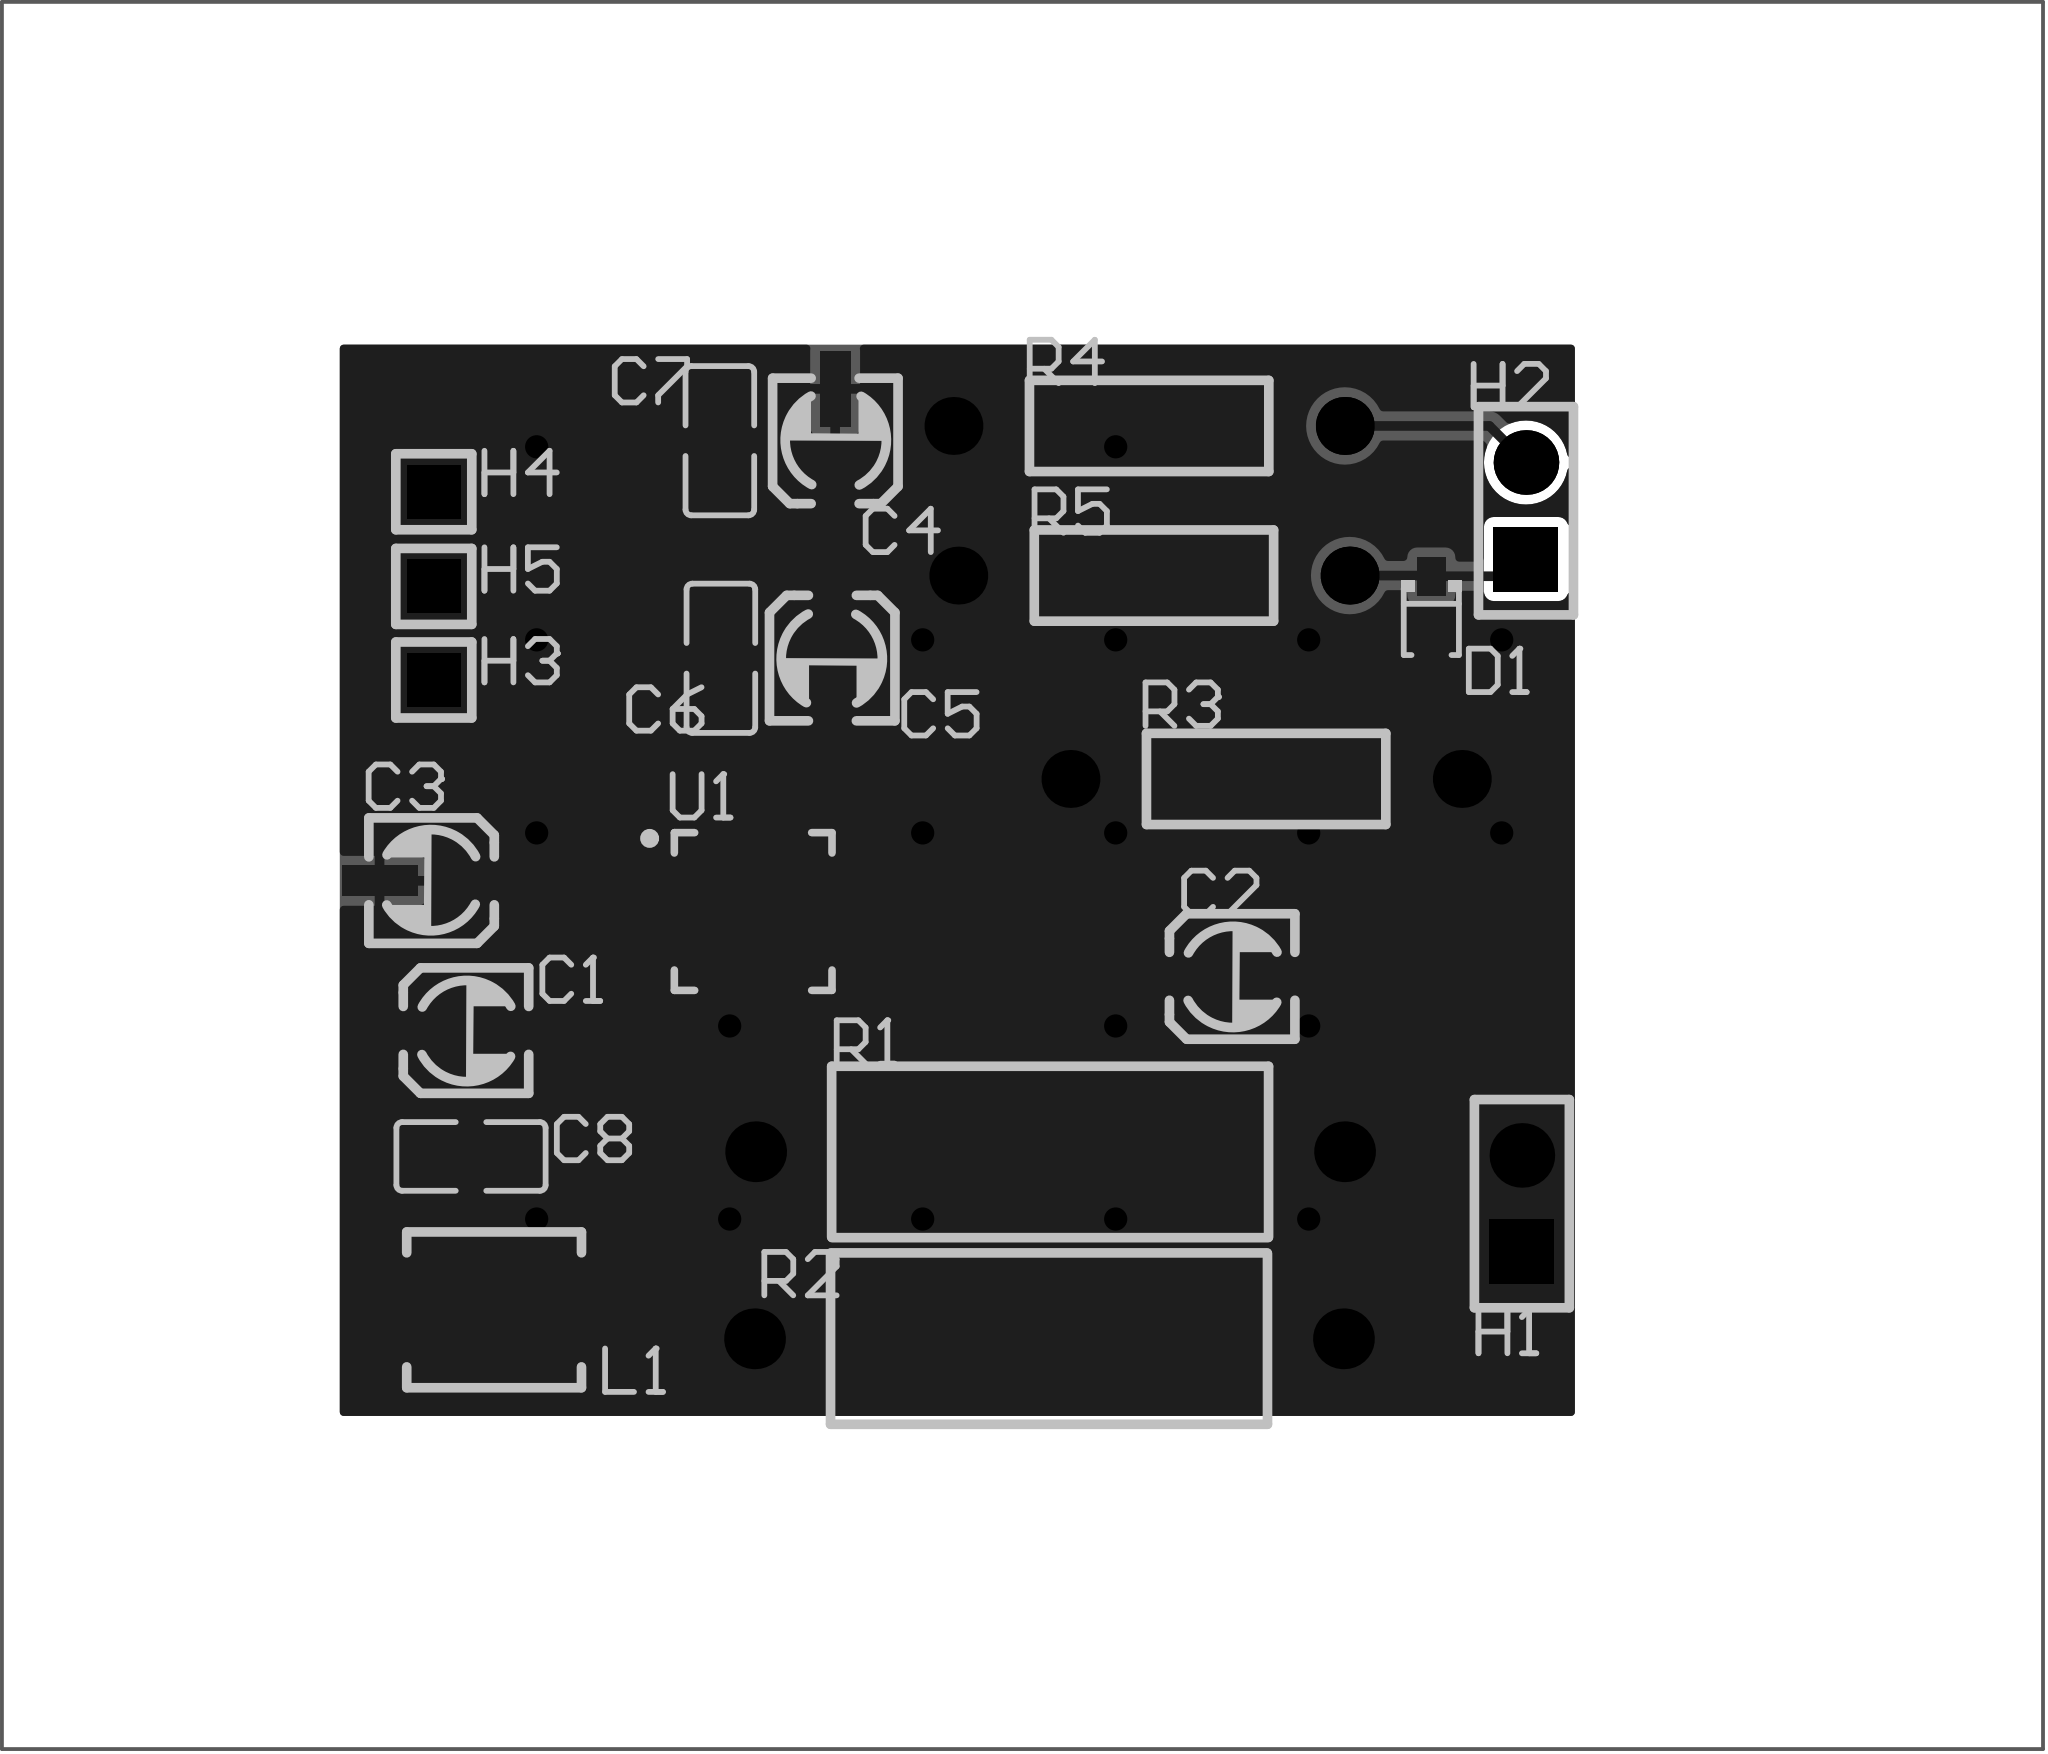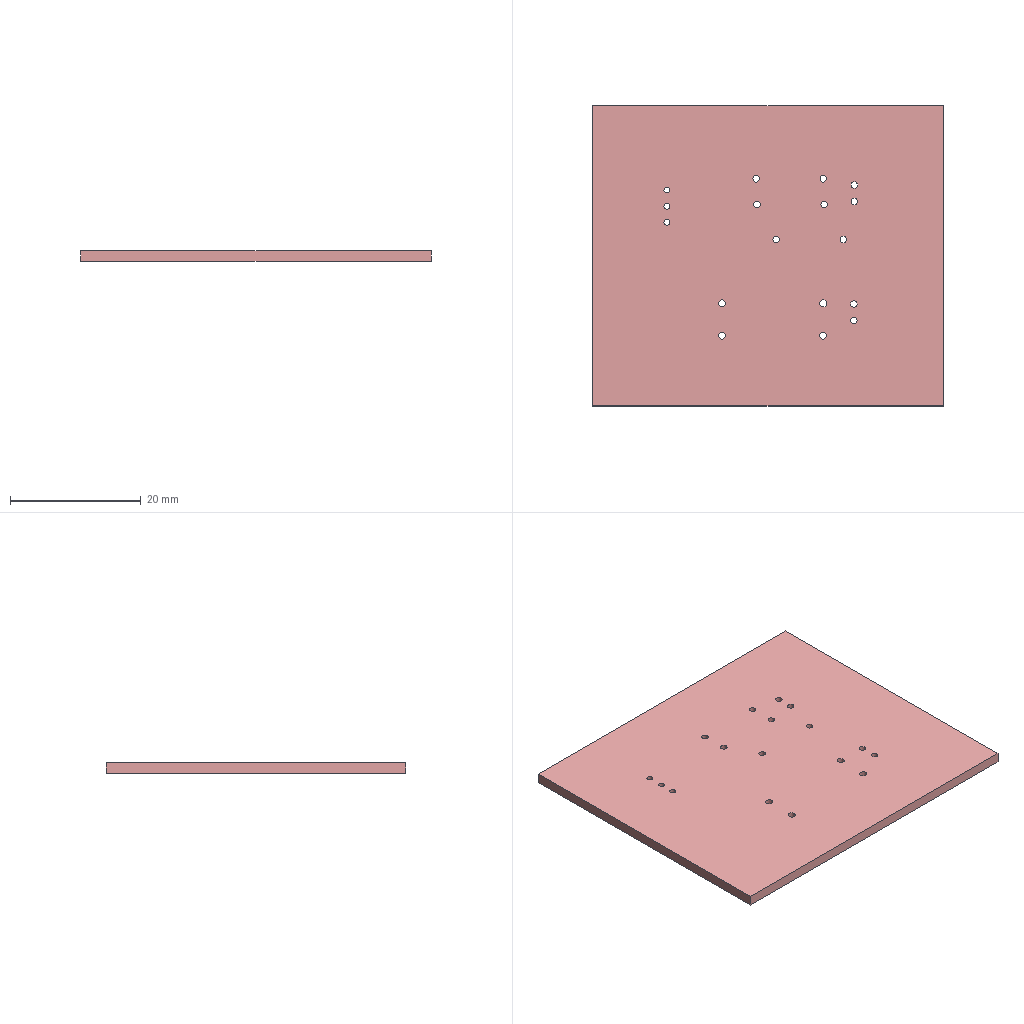Circuit board layout | Altium Designer | box 53.7 x 46 x 1.6 mm
Layer stack:
# Altium Designer layer stack of  (unit mm; dielectric type: 0 none, 1 core, 2 prepreg, 3 surface material)
index,name,kind,layer,copper_thickness_mm,dielectric_type,dielectric_thickness_mm,dielectric_material,dielectric_constant
0,Top Paste Mask Layer,other,,,,,,
1,Top Silkscreen Layer,other,,,,,,
2,Top Solder Mask Layer,dielectric,,,3,0.01,,3.3
3,Top Layer,copper,Top Layer,0.035,,,,
4,Dielectric1,dielectric,,,3,1.51,FR4,4.5
5,Bottom Layer,copper,Bottom Layer,0.035,,,,
6,Bottom Solder Mask Layer,dielectric,,,3,0.01,,3.3
7,Bottom Silkscreen Layer,other,,,,,,
8,Bottom Paste Mask Layer,other,,,,,,
# drill layer pairs: low layer,high layer
drill_pair,Top Layer,Bottom Layer
Part placement:
Designator,Comment,Layer,Footprint,Center-X(mm),Center-Y(mm),Rotation
C1,0.1uF,TopLayer,C_Ele_SMD_3x5.4mm,82.064,88.76,180
C2,100nF/250V,TopLayer,C_Ele_SMD_3x5.4mm,102.23,90.184,180
C3,0.1u,TopLayer,C_Ele_SMD_3x5.4mm,81.158,92.696,0
C4,10nF,TopLayer,C_Ele_SMD_3x5.4mm,91.78,104.272,270
C5,10nF,TopLayer,C_Ele_SMD_3x5.4mm,91.708,98.557,90
C6,100nF,TopLayer,C0805,88.773,98.552,90
C7,100nF,TopLayer,C0805,88.746,104.277,270
C8,10u,TopLayer,C0805,82.196,85.444,180
D1,BAT165E6327,TopLayer,SOD-323_L1.8-W1.3-LS2.5-RD,107.472,99.538,270
H1,,TopLayer,HDR-TH_2P-P2.54-V-F,109.855,84.201,90
H2,,TopLayer,HDR-TH_2P-P2.54-V-F,109.963,102.434,90
H3,,TopLayer,HDR-TH_1P-V-M_XKB_X4611WV-01I-C28D40,81.217,97.981,180
H4,,TopLayer,HDR-TH_1P-V-M_XKB_X4611WV-01I-C28D40,81.217,102.934,180
H5,,TopLayer,HDR-TH_1P-V-M_XKB_X4611WV-01I-C28D40,81.216,100.443,180
L1,4.7uH,TopLayer,IND-SMD_L4.6-W4.1-A,82.804,81.407,0
R1,1.72M,TopLayer,Res_1W,97.438,85.567,0
R2,15k,TopLayer,Res_1W,97.409,80.645,180
R3,18k,TopLayer,Res_1/4W,103.124,95.377,180
R4,1k,TopLayer,Res_1/4W,100.044,104.666,180
R5,1k,TopLayer,Res_1/4W,100.171,100.729,180
U1,DRV2700,TopLayer,TI-RGP20-2700X2700TP_V,89.623,91.889,0
Pad and via stacks:
# Altium Designer via and pad stacks of  (unit mm). Each distinct definition once, with the count of objects using it.
# via: kind,start_layer,end_layer,hole_mm,diameter_mm,mode(0 simple;1 top-mid-bottom;2 full stack),diameter_per_layer,count,example_net
# pad: kind,layer,hole_mm,hole_type(0 round;1 square;2 slot),plating,top_size,top_shape(1 round;2 rect;3 octagon;9 rounded rect),mid_size,bottom_size,mode,footprint,size_per_layer,count,example
pad,Top Layer,0,0,plated,1.999x0.8001,2,1.999x0.8001,1.999x0.8001,0,C_Ele_SMD_3x5.4mm,,10,C1.1
pad,Top Layer,0,0,plated,1.41x1.35,2,1.41x1.35,1.41x1.35,0,C0805,,6,C6.2
pad,Top Layer,0,0,plated,1x0.75,2,1x0.75,1x0.75,0,SOD-323_L1.8-W1.3-LS2.5-RD,,2,D1.2
pad,Top Layer,0,0,plated,2.5x1.5,2,2.5x1.5,2.5x1.5,0,IND-SMD_L4.6-W4.1-A,,2,L1.1
pad,Top Layer,0,0,plated,2.705x2.705,2,2.705x2.705,2.705x2.705,0,TI-RGP20-2700X2700TP_V,,1,U1.21
pad,Top Layer,0,0,plated,0.2921x0.8763,2,0.2921x0.8763,0.2921x0.8763,0,TI-RGP20-2700X2700TP_V,,20,U1.20
pad,Multi-Layer,1,0,plated,1.7x1.7,2,1.7x1.7,1.7x1.7,0,HDR-TH_2P-P2.54-V-F,,2,H1.1
pad,Multi-Layer,1,0,plated,1.7x1.7,1,1.7x1.7,1.7x1.7,0,HDR-TH_2P-P2.54-V-F,,2,H1.2
pad,Multi-Layer,0.9,0,plated,1.4x1.4,2,1.4x1.4,1.4x1.4,0,HDR-TH_1P-V-M_XKB_X4611WV-01I-C28D40,,3,H3.1
pad,Multi-Layer,1.1,0,plated,1.6x1.6,1,1.6x1.6,1.6x1.6,0,Res_1W,,4,R1.1
pad,Multi-Layer,1,0,plated,1.524x1.524,1,1.524x1.524,1.524x1.524,0,Res_1/4W,,6,R3.1
via,Top Layer,Bottom Layer,0.2997,0.5004,0,,9,GND
via,Top Layer,Bottom Layer,0.3048,0.61,0,,20,GND
Copper pours:
name,layer,net,type(0 solid;1 hatched;2 none)
Top Layer-GND,Top Layer,GND,0
Bottom Layer-GND,Bottom Layer,GND,0
Design rules, without the lines most boards share:
# Altium Designer design rules of  (exported by Altium Designer, unit mm)
# columns: name | kind | enabled | priority | scope1 | scope2 | descriptor | typed fields (field=value)
copperRegion | 20 | enabled | 1 | (InNet('GND')) | All | Polygon Connect Rule(Relief Connect )(Conductor Width=10mil) (Relief Angle=90 Angle) (Entries=4) (Air Gap Width=10mil) ((InNet('GND'))),(All) | connect_style(0=relief,1=direct,2=none)=0 relief_conductor_width=0.254 relief_entries=4